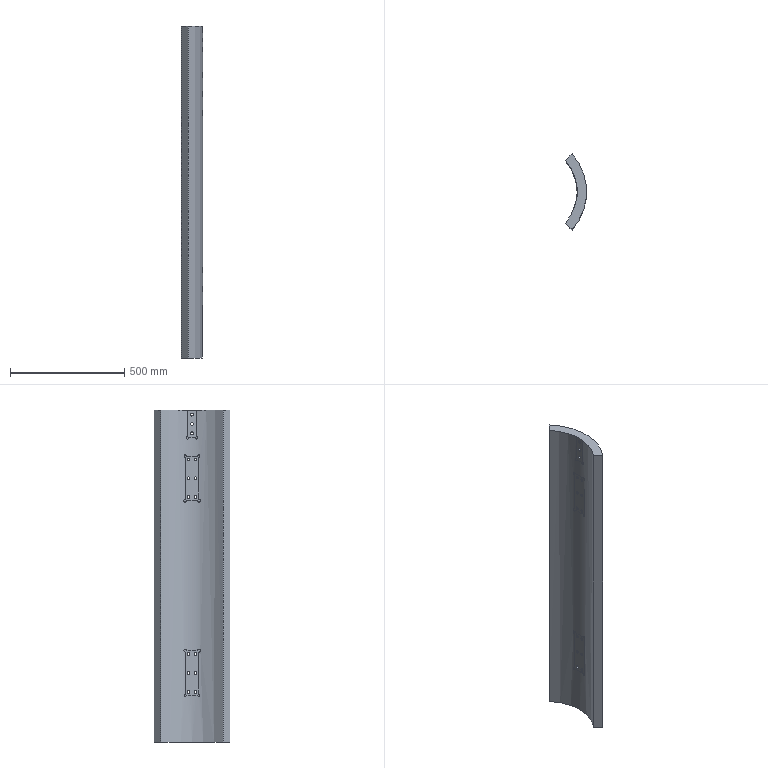Part | SolidWorks | features BaseBody 1 | 1 solid | 115 faces | box 91.989 x 331.703 x 1450 mm | volume 19488454 mm3 | cylinder 77 | plane 38 | commonest cylinder face diameters 12.5 x30 22 x26 10.571 x4 12.179 x4 10 x3 10.162 x2